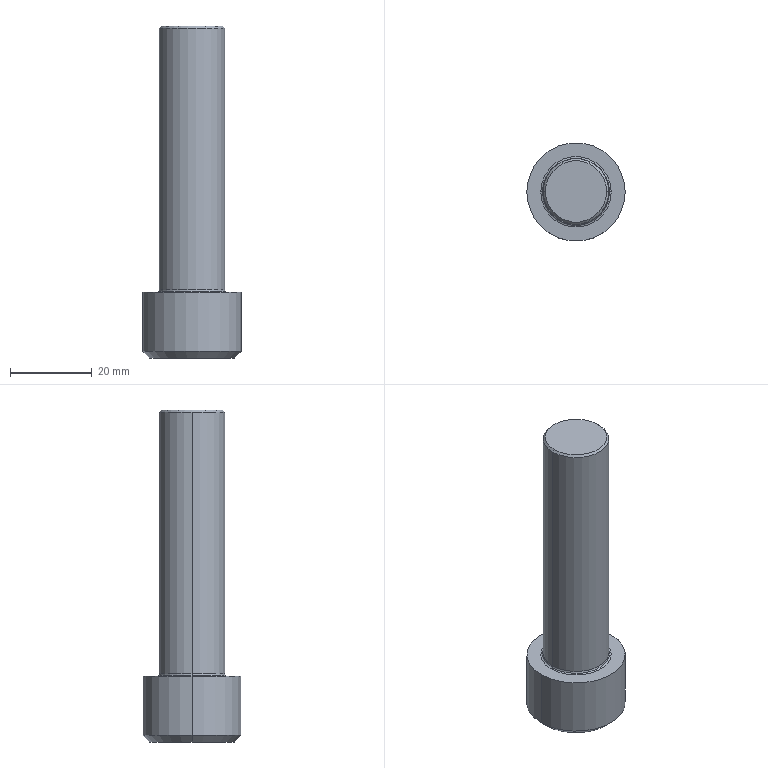Part | Creo | 1 solid | 23 faces | box 24 x 24 x 81 mm | volume 18544 mm3 | plane 9 | cone 6 | cylinder 4 | torus 4 | commonest cylinder face diameters 16 x2 24 x2
STEP:
#1=CARTESIAN_POINT('',(0.,0.,0.));
#2=DIRECTION('',(0.,0.,1.));
#3=DIRECTION('',(1.,0.,0.));
#4=AXIS2_PLACEMENT_3D('',#1,#2,#3);
#5=CARTESIAN_POINT('',(91.917,-8.,72.172));
#6=VERTEX_POINT('',#5);
#7=CARTESIAN_POINT('',(95.959,-1.,72.172));
#8=VERTEX_POINT('',#7);
#9=CARTESIAN_POINT('',(91.917,-8.,72.172));
#10=CARTESIAN_POINT('',(92.106,-7.673,72.281));
#11=CARTESIAN_POINT('',(92.484,-7.018,72.477));
#12=CARTESIAN_POINT('',(93.06,-6.021,72.689));
#13=CARTESIAN_POINT('',(93.642,-5.012,72.802));
#14=CARTESIAN_POINT('',(94.231,-3.992,72.802));
#15=CARTESIAN_POINT('',(94.814,-2.982,72.69));
#16=CARTESIAN_POINT('',(95.39,-1.986,72.478));
#17=CARTESIAN_POINT('',(95.769,-1.328,72.282));
#18=CARTESIAN_POINT('',(95.959,-1.,72.172));
#19=B_SPLINE_CURVE_WITH_KNOTS('',3,(#9,#10,#11,#12,#13,#14,#15,#16,#17,#18),.UNSPECIFIED.,.F.,.F.,(4,1,1,1,1,1,1,4),(0.,0.1429,0.2857,0.4286,0.5714,0.7143,0.8571,1.),.UNSPECIFIED.);
#20=EDGE_CURVE('',#6,#8,#19,.T.);
#21=ORIENTED_EDGE('',*,*,#20,.F.);
#22=CARTESIAN_POINT('',(100.,-8.,76.839));
#23=VERTEX_POINT('',#22);
#24=CARTESIAN_POINT('',(100.,-8.,76.839));
#25=DIRECTION('',(-0.866,0.,-0.5));
#26=VECTOR('',#25,9.333);
#27=LINE('',#24,#26);
#28=EDGE_CURVE('',#23,#6,#27,.T.);
#29=ORIENTED_EDGE('',*,*,#28,.F.);
#30=CARTESIAN_POINT('',(108.083,-8.,72.172));
#31=VERTEX_POINT('',#30);
#32=CARTESIAN_POINT('',(100.,-8.,76.839));
#33=DIRECTION('',(0.866,0.,-0.5));
#34=VECTOR('',#33,9.333);
#35=LINE('',#32,#34);
#36=EDGE_CURVE('',#23,#31,#35,.T.);
#37=ORIENTED_EDGE('',*,*,#36,.T.);
#38=CARTESIAN_POINT('',(104.041,-1.,72.172));
#39=VERTEX_POINT('',#38);
#40=CARTESIAN_POINT('',(104.041,-1.,72.172));
#41=CARTESIAN_POINT('',(104.23,-1.327,72.281));
#42=CARTESIAN_POINT('',(104.609,-1.982,72.477));
#43=CARTESIAN_POINT('',(105.184,-2.979,72.689));
#44=CARTESIAN_POINT('',(105.767,-3.988,72.802));
#45=CARTESIAN_POINT('',(106.356,-5.008,72.802));
#46=CARTESIAN_POINT('',(106.939,-6.018,72.69));
#47=CARTESIAN_POINT('',(107.514,-7.014,72.478));
#48=CARTESIAN_POINT('',(107.894,-7.672,72.282));
#49=CARTESIAN_POINT('',(108.083,-8.,72.172));
#50=B_SPLINE_CURVE_WITH_KNOTS('',3,(#40,#41,#42,#43,#44,#45,#46,#47,#48,#49),.UNSPECIFIED.,.F.,.F.,(4,1,1,1,1,1,1,4),(0.,0.1429,0.2857,0.4286,0.5714,0.7143,0.8571,1.),.UNSPECIFIED.);
#51=EDGE_CURVE('',#39,#31,#50,.T.);
#52=ORIENTED_EDGE('',*,*,#51,.F.);
#53=CARTESIAN_POINT('',(95.959,-1.,72.172));
#54=CARTESIAN_POINT('',(96.333,-1.,72.281));
#55=CARTESIAN_POINT('',(97.086,-1.,72.476));
#56=CARTESIAN_POINT('',(98.244,-1.,72.69));
#57=CARTESIAN_POINT('',(99.413,-1.,72.802));
#58=CARTESIAN_POINT('',(100.583,-1.,72.802));
#59=CARTESIAN_POINT('',(101.75,-1.,72.69));
#60=CARTESIAN_POINT('',(102.908,-1.,72.477));
#61=CARTESIAN_POINT('',(103.665,-1.,72.281));
#62=CARTESIAN_POINT('',(104.041,-1.,72.172));
#63=B_SPLINE_CURVE_WITH_KNOTS('',3,(#53,#54,#55,#56,#57,#58,#59,#60,#61,#62),.UNSPECIFIED.,.F.,.F.,(4,1,1,1,1,1,1,4),(0.,0.1429,0.2857,0.4286,0.5714,0.7143,0.8571,1.),.UNSPECIFIED.);
#64=EDGE_CURVE('',#8,#39,#63,.T.);
#65=ORIENTED_EDGE('',*,*,#64,.F.);
#66=EDGE_LOOP('',(#21,#29,#37,#52,#65));
#67=FACE_OUTER_BOUND('',#66,.F.);
#68=CARTESIAN_POINT('',(100.,-8.,74.459));
#69=DIRECTION('',(0.,0.,-1.));
#70=DIRECTION('',(-1.,0.,0.));
#71=AXIS2_PLACEMENT_3D('',#68,#69,#70);
#72=CONICAL_SURFACE('',#71,4.122,60.);
#73=ADVANCED_FACE('',(#67),#72,.F.);
#74=CARTESIAN_POINT('',(95.959,-1.,64.172));
#75=VERTEX_POINT('',#74);
#76=CARTESIAN_POINT('',(91.917,-8.,64.172));
#77=VERTEX_POINT('',#76);
#78=CARTESIAN_POINT('',(95.959,-1.,64.172));
#79=DIRECTION('',(-0.5,-0.866,0.));
#80=VECTOR('',#79,8.083);
#81=LINE('',#78,#80);
#82=EDGE_CURVE('',#75,#77,#81,.T.);
#83=ORIENTED_EDGE('',*,*,#82,.T.);
#84=CARTESIAN_POINT('',(91.917,-8.,64.172));
#85=DIRECTION('',(0.,0.,1.));
#86=VECTOR('',#85,8.);
#87=LINE('',#84,#86);
#88=EDGE_CURVE('',#77,#6,#87,.T.);
#89=ORIENTED_EDGE('',*,*,#88,.T.);
#90=ORIENTED_EDGE('',*,*,#20,.T.);
#91=CARTESIAN_POINT('',(95.959,-1.,64.172));
#92=DIRECTION('',(0.,0.,1.));
#93=VECTOR('',#92,8.);
#94=LINE('',#91,#93);
#95=EDGE_CURVE('',#75,#8,#94,.T.);
#96=ORIENTED_EDGE('',*,*,#95,.F.);
#97=EDGE_LOOP('',(#83,#89,#90,#96));
#98=FACE_OUTER_BOUND('',#97,.F.);
#99=CARTESIAN_POINT('',(95.959,-1.,72.172));
#100=DIRECTION('',(0.866,-0.5,0.));
#101=DIRECTION('',(-0.5,-0.866,0.));
#102=AXIS2_PLACEMENT_3D('',#99,#100,#101);
#103=PLANE('',#102);
#104=ADVANCED_FACE('',(#98),#103,.T.);
#105=CARTESIAN_POINT('',(89.6,-8.,64.172));
#106=VERTEX_POINT('',#105);
#107=CARTESIAN_POINT('',(110.4,-8.,64.172));
#108=VERTEX_POINT('',#107);
#109=CARTESIAN_POINT('',(100.,-8.,64.172));
#110=DIRECTION('',(0.,0.,-1.));
#111=DIRECTION('',(-1.,0.,0.));
#112=AXIS2_PLACEMENT_3D('',#109,#110,#111);
#113=CIRCLE('',#112,10.4);
#114=EDGE_CURVE('',#106,#108,#113,.T.);
#115=ORIENTED_EDGE('',*,*,#114,.F.);
#116=CARTESIAN_POINT('',(100.,-8.,64.172));
#117=DIRECTION('',(0.,0.,-1.));
#118=DIRECTION('',(1.,0.,0.));
#119=AXIS2_PLACEMENT_3D('',#116,#117,#118);
#120=CIRCLE('',#119,10.4);
#121=EDGE_CURVE('',#108,#106,#120,.T.);
#122=ORIENTED_EDGE('',*,*,#121,.F.);
#123=EDGE_LOOP('',(#115,#122));
#124=FACE_OUTER_BOUND('',#123,.F.);
#125=CARTESIAN_POINT('',(95.959,-15.,64.172));
#126=VERTEX_POINT('',#125);
#127=CARTESIAN_POINT('',(91.917,-8.,64.172));
#128=DIRECTION('',(0.5,-0.866,0.));
#129=VECTOR('',#128,8.083);
#130=LINE('',#127,#129);
#131=EDGE_CURVE('',#77,#126,#130,.T.);
#132=ORIENTED_EDGE('',*,*,#131,.F.);
#133=ORIENTED_EDGE('',*,*,#82,.F.);
#134=CARTESIAN_POINT('',(104.041,-1.,64.172));
#135=VERTEX_POINT('',#134);
#136=CARTESIAN_POINT('',(95.959,-1.,64.172));
#137=DIRECTION('',(1.,0.,0.));
#138=VECTOR('',#137,8.083);
#139=LINE('',#136,#138);
#140=EDGE_CURVE('',#75,#135,#139,.T.);
#141=ORIENTED_EDGE('',*,*,#140,.T.);
#142=CARTESIAN_POINT('',(108.083,-8.,64.172));
#143=VERTEX_POINT('',#142);
#144=CARTESIAN_POINT('',(108.083,-8.,64.172));
#145=DIRECTION('',(-0.5,0.866,0.));
#146=VECTOR('',#145,8.083);
#147=LINE('',#144,#146);
#148=EDGE_CURVE('',#143,#135,#147,.T.);
#149=ORIENTED_EDGE('',*,*,#148,.F.);
#150=CARTESIAN_POINT('',(104.041,-15.,64.172));
#151=VERTEX_POINT('',#150);
#152=CARTESIAN_POINT('',(104.041,-15.,64.172));
#153=DIRECTION('',(0.5,0.866,0.));
#154=VECTOR('',#153,8.083);
#155=LINE('',#152,#154);
#156=EDGE_CURVE('',#151,#143,#155,.T.);
#157=ORIENTED_EDGE('',*,*,#156,.F.);
#158=CARTESIAN_POINT('',(104.041,-15.,64.172));
#159=DIRECTION('',(-1.,0.,0.));
#160=VECTOR('',#159,8.083);
#161=LINE('',#158,#160);
#162=EDGE_CURVE('',#151,#126,#161,.T.);
#163=ORIENTED_EDGE('',*,*,#162,.T.);
#164=EDGE_LOOP('',(#132,#133,#141,#149,#157,#163));
#165=FACE_BOUND('',#164,.F.);
#166=CARTESIAN_POINT('',(100.,-8.,64.172));
#167=DIRECTION('',(0.,0.,-1.));
#168=DIRECTION('',(-1.,0.,0.));
#169=AXIS2_PLACEMENT_3D('',#166,#167,#168);
#170=PLANE('',#169);
#171=ADVANCED_FACE('',(#124,#165),#170,.T.);
#172=CARTESIAN_POINT('',(88.,-8.,65.772));
#173=VERTEX_POINT('',#172);
#174=CARTESIAN_POINT('',(112.,-8.,65.772));
#175=VERTEX_POINT('',#174);
#176=CARTESIAN_POINT('',(100.,-8.,65.772));
#177=DIRECTION('',(0.,0.,-1.));
#178=DIRECTION('',(-1.,0.,0.));
#179=AXIS2_PLACEMENT_3D('',#176,#177,#178);
#180=CIRCLE('',#179,12.);
#181=EDGE_CURVE('',#173,#175,#180,.T.);
#182=ORIENTED_EDGE('',*,*,#181,.F.);
#183=CARTESIAN_POINT('',(89.6,-8.,64.172));
#184=DIRECTION('',(-0.7071,0.,0.7071));
#185=VECTOR('',#184,2.263);
#186=LINE('',#183,#185);
#187=EDGE_CURVE('',#106,#173,#186,.T.);
#188=ORIENTED_EDGE('',*,*,#187,.F.);
#189=ORIENTED_EDGE('',*,*,#114,.T.);
#190=CARTESIAN_POINT('',(110.4,-8.,64.172));
#191=DIRECTION('',(0.7071,0.,0.7071));
#192=VECTOR('',#191,2.263);
#193=LINE('',#190,#192);
#194=EDGE_CURVE('',#108,#175,#193,.T.);
#195=ORIENTED_EDGE('',*,*,#194,.T.);
#196=EDGE_LOOP('',(#182,#188,#189,#195));
#197=FACE_OUTER_BOUND('',#196,.F.);
#198=CARTESIAN_POINT('',(100.,-8.,64.972));
#199=DIRECTION('',(0.,0.,1.));
#200=DIRECTION('',(1.,0.,0.));
#201=AXIS2_PLACEMENT_3D('',#198,#199,#200);
#202=CONICAL_SURFACE('',#201,11.2,45.);
#203=ADVANCED_FACE('',(#197),#202,.T.);
#204=ORIENTED_EDGE('',*,*,#181,.T.);
#205=CARTESIAN_POINT('',(112.,-8.,80.172));
#206=VERTEX_POINT('',#205);
#207=CARTESIAN_POINT('',(112.,-8.,80.172));
#208=DIRECTION('',(0.,0.,-1.));
#209=VECTOR('',#208,14.4);
#210=LINE('',#207,#209);
#211=EDGE_CURVE('',#206,#175,#210,.T.);
#212=ORIENTED_EDGE('',*,*,#211,.F.);
#213=CARTESIAN_POINT('',(88.,-8.,80.172));
#214=VERTEX_POINT('',#213);
#215=CARTESIAN_POINT('',(100.,-8.,80.172));
#216=DIRECTION('',(0.,0.,1.));
#217=DIRECTION('',(1.,0.,0.));
#218=AXIS2_PLACEMENT_3D('',#215,#216,#217);
#219=CIRCLE('',#218,12.);
#220=EDGE_CURVE('',#206,#214,#219,.T.);
#221=ORIENTED_EDGE('',*,*,#220,.T.);
#222=CARTESIAN_POINT('',(88.,-8.,80.172));
#223=DIRECTION('',(0.,0.,-1.));
#224=VECTOR('',#223,14.4);
#225=LINE('',#222,#224);
#226=EDGE_CURVE('',#214,#173,#225,.T.);
#227=ORIENTED_EDGE('',*,*,#226,.T.);
#228=EDGE_LOOP('',(#204,#212,#221,#227));
#229=FACE_OUTER_BOUND('',#228,.F.);
#230=CARTESIAN_POINT('',(100.,-8.,80.172));
#231=DIRECTION('',(0.,0.,-1.));
#232=DIRECTION('',(-1.,0.,0.));
#233=AXIS2_PLACEMENT_3D('',#230,#231,#232);
#234=CYLINDRICAL_SURFACE('',#233,12.);
#235=ADVANCED_FACE('',(#229),#234,.T.);
#236=CARTESIAN_POINT('',(100.,-8.,65.772));
#237=DIRECTION('',(0.,0.,-1.));
#238=DIRECTION('',(1.,0.,0.));
#239=AXIS2_PLACEMENT_3D('',#236,#237,#238);
#240=CIRCLE('',#239,12.);
#241=EDGE_CURVE('',#175,#173,#240,.T.);
#242=ORIENTED_EDGE('',*,*,#241,.T.);
#243=ORIENTED_EDGE('',*,*,#226,.F.);
#244=CARTESIAN_POINT('',(100.,-8.,80.172));
#245=DIRECTION('',(0.,0.,1.));
#246=DIRECTION('',(-1.,0.,0.));
#247=AXIS2_PLACEMENT_3D('',#244,#245,#246);
#248=CIRCLE('',#247,12.);
#249=EDGE_CURVE('',#214,#206,#248,.T.);
#250=ORIENTED_EDGE('',*,*,#249,.T.);
#251=ORIENTED_EDGE('',*,*,#211,.T.);
#252=EDGE_LOOP('',(#242,#243,#250,#251));
#253=FACE_OUTER_BOUND('',#252,.F.);
#254=CARTESIAN_POINT('',(100.,-8.,80.172));
#255=DIRECTION('',(0.,0.,-1.));
#256=DIRECTION('',(-1.,0.,0.));
#257=AXIS2_PLACEMENT_3D('',#254,#255,#256);
#258=CYLINDRICAL_SURFACE('',#257,12.);
#259=ADVANCED_FACE('',(#253),#258,.T.);
#260=ORIENTED_EDGE('',*,*,#241,.F.);
#261=ORIENTED_EDGE('',*,*,#194,.F.);
#262=ORIENTED_EDGE('',*,*,#121,.T.);
#263=ORIENTED_EDGE('',*,*,#187,.T.);
#264=EDGE_LOOP('',(#260,#261,#262,#263));
#265=FACE_OUTER_BOUND('',#264,.F.);
#266=CARTESIAN_POINT('',(100.,-8.,64.972));
#267=DIRECTION('',(0.,0.,1.));
#268=DIRECTION('',(1.,0.,0.));
#269=AXIS2_PLACEMENT_3D('',#266,#267,#268);
#270=CONICAL_SURFACE('',#269,11.2,45.);
#271=ADVANCED_FACE('',(#265),#270,.T.);
#272=ORIENTED_EDGE('',*,*,#249,.F.);
#273=ORIENTED_EDGE('',*,*,#220,.F.);
#274=EDGE_LOOP('',(#272,#273));
#275=FACE_OUTER_BOUND('',#274,.F.);
#276=CARTESIAN_POINT('',(91.4,-8.,80.172));
#277=VERTEX_POINT('',#276);
#278=CARTESIAN_POINT('',(108.6,-8.,80.172));
#279=VERTEX_POINT('',#278);
#280=CARTESIAN_POINT('',(100.,-8.,80.172));
#281=DIRECTION('',(0.,0.,-1.));
#282=DIRECTION('',(-1.,0.,0.));
#283=AXIS2_PLACEMENT_3D('',#280,#281,#282);
#284=CIRCLE('',#283,8.6);
#285=EDGE_CURVE('',#277,#279,#284,.T.);
#286=ORIENTED_EDGE('',*,*,#285,.F.);
#287=CARTESIAN_POINT('',(100.,-8.,80.172));
#288=DIRECTION('',(0.,0.,-1.));
#289=DIRECTION('',(1.,0.,0.));
#290=AXIS2_PLACEMENT_3D('',#287,#288,#289);
#291=CIRCLE('',#290,8.6);
#292=EDGE_CURVE('',#279,#277,#291,.T.);
#293=ORIENTED_EDGE('',*,*,#292,.F.);
#294=EDGE_LOOP('',(#286,#293));
#295=FACE_BOUND('',#294,.F.);
#296=CARTESIAN_POINT('',(100.,-8.,80.172));
#297=DIRECTION('',(0.,0.,-1.));
#298=DIRECTION('',(-1.,0.,0.));
#299=AXIS2_PLACEMENT_3D('',#296,#297,#298);
#300=PLANE('',#299);
#301=ADVANCED_FACE('',(#275,#295),#300,.F.);
#302=ORIENTED_EDGE('',*,*,#285,.T.);
#303=CARTESIAN_POINT('',(108.176,-8.,80.348));
#304=VERTEX_POINT('',#303);
#305=CARTESIAN_POINT('',(108.6,-8.,80.772));
#306=DIRECTION('',(0.,1.,0.));
#307=DIRECTION('',(0.,0.,-1.));
#308=AXIS2_PLACEMENT_3D('',#305,#306,#307);
#309=CIRCLE('',#308,0.6);
#310=EDGE_CURVE('',#279,#304,#309,.T.);
#311=ORIENTED_EDGE('',*,*,#310,.T.);
#312=CARTESIAN_POINT('',(91.824,-8.,80.348));
#313=VERTEX_POINT('',#312);
#314=CARTESIAN_POINT('',(100.,-8.,80.348));
#315=DIRECTION('',(0.,0.,-1.));
#316=DIRECTION('',(-1.,0.,0.));
#317=AXIS2_PLACEMENT_3D('',#314,#315,#316);
#318=CIRCLE('',#317,8.176);
#319=EDGE_CURVE('',#313,#304,#318,.T.);
#320=ORIENTED_EDGE('',*,*,#319,.F.);
#321=CARTESIAN_POINT('',(91.4,-8.,80.772));
#322=DIRECTION('',(0.,-1.,0.));
#323=DIRECTION('',(0.,0.,-1.));
#324=AXIS2_PLACEMENT_3D('',#321,#322,#323);
#325=CIRCLE('',#324,0.6);
#326=EDGE_CURVE('',#277,#313,#325,.T.);
#327=ORIENTED_EDGE('',*,*,#326,.F.);
#328=EDGE_LOOP('',(#302,#311,#320,#327));
#329=FACE_OUTER_BOUND('',#328,.F.);
#330=CARTESIAN_POINT('',(100.,-8.,80.772));
#331=DIRECTION('',(0.,0.,-1.));
#332=DIRECTION('',(-1.,0.,0.));
#333=AXIS2_PLACEMENT_3D('',#330,#331,#332);
#334=TOROIDAL_SURFACE('',#333,8.6,0.6);
#335=ADVANCED_FACE('',(#329),#334,.F.);
#336=ORIENTED_EDGE('',*,*,#292,.T.);
#337=ORIENTED_EDGE('',*,*,#326,.T.);
#338=CARTESIAN_POINT('',(100.,-8.,80.348));
#339=DIRECTION('',(0.,0.,-1.));
#340=DIRECTION('',(1.,0.,0.));
#341=AXIS2_PLACEMENT_3D('',#338,#339,#340);
#342=CIRCLE('',#341,8.176);
#343=EDGE_CURVE('',#304,#313,#342,.T.);
#344=ORIENTED_EDGE('',*,*,#343,.F.);
#345=ORIENTED_EDGE('',*,*,#310,.F.);
#346=EDGE_LOOP('',(#336,#337,#344,#345));
#347=FACE_OUTER_BOUND('',#346,.F.);
#348=CARTESIAN_POINT('',(100.,-8.,80.772));
#349=DIRECTION('',(0.,0.,-1.));
#350=DIRECTION('',(-1.,0.,0.));
#351=AXIS2_PLACEMENT_3D('',#348,#349,#350);
#352=TOROIDAL_SURFACE('',#351,8.6,0.6);
#353=ADVANCED_FACE('',(#347),#352,.F.);
#354=CARTESIAN_POINT('',(108.,-8.,80.772));
#355=VERTEX_POINT('',#354);
#356=CARTESIAN_POINT('',(92.,-8.,80.772));
#357=VERTEX_POINT('',#356);
#358=CARTESIAN_POINT('',(100.,-8.,80.772));
#359=DIRECTION('',(0.,0.,-1.));
#360=DIRECTION('',(1.,0.,0.));
#361=AXIS2_PLACEMENT_3D('',#358,#359,#360);
#362=CIRCLE('',#361,8.);
#363=EDGE_CURVE('',#355,#357,#362,.T.);
#364=ORIENTED_EDGE('',*,*,#363,.F.);
#365=CARTESIAN_POINT('',(108.6,-8.,80.772));
#366=DIRECTION('',(0.,1.,0.));
#367=DIRECTION('',(-0.7071,0.,-0.7071));
#368=AXIS2_PLACEMENT_3D('',#365,#366,#367);
#369=CIRCLE('',#368,0.6);
#370=EDGE_CURVE('',#304,#355,#369,.T.);
#371=ORIENTED_EDGE('',*,*,#370,.F.);
#372=ORIENTED_EDGE('',*,*,#343,.T.);
#373=CARTESIAN_POINT('',(91.4,-8.,80.772));
#374=DIRECTION('',(0.,-1.,0.));
#375=DIRECTION('',(0.7071,0.,-0.7071));
#376=AXIS2_PLACEMENT_3D('',#373,#374,#375);
#377=CIRCLE('',#376,0.6);
#378=EDGE_CURVE('',#313,#357,#377,.T.);
#379=ORIENTED_EDGE('',*,*,#378,.T.);
#380=EDGE_LOOP('',(#364,#371,#372,#379));
#381=FACE_OUTER_BOUND('',#380,.F.);
#382=CARTESIAN_POINT('',(100.,-8.,80.772));
#383=DIRECTION('',(0.,0.,-1.));
#384=DIRECTION('',(-1.,0.,0.));
#385=AXIS2_PLACEMENT_3D('',#382,#383,#384);
#386=TOROIDAL_SURFACE('',#385,8.6,0.6);
#387=ADVANCED_FACE('',(#381),#386,.F.);
#388=CARTESIAN_POINT('',(92.,-8.,144.673));
#389=VERTEX_POINT('',#388);
#390=CARTESIAN_POINT('',(108.,-8.,144.673));
#391=VERTEX_POINT('',#390);
#392=CARTESIAN_POINT('',(100.,-8.,144.673));
#393=DIRECTION('',(0.,0.,1.));
#394=DIRECTION('',(-1.,0.,0.));
#395=AXIS2_PLACEMENT_3D('',#392,#393,#394);
#396=CIRCLE('',#395,8.);
#397=EDGE_CURVE('',#389,#391,#396,.T.);
#398=ORIENTED_EDGE('',*,*,#397,.T.);
#399=CARTESIAN_POINT('',(108.,-8.,144.673));
#400=DIRECTION('',(0.,0.,-1.));
#401=VECTOR('',#400,63.9);
#402=LINE('',#399,#401);
#403=EDGE_CURVE('',#391,#355,#402,.T.);
#404=ORIENTED_EDGE('',*,*,#403,.T.);
#405=ORIENTED_EDGE('',*,*,#363,.T.);
#406=CARTESIAN_POINT('',(92.,-8.,144.673));
#407=DIRECTION('',(0.,0.,-1.));
#408=VECTOR('',#407,63.9);
#409=LINE('',#406,#408);
#410=EDGE_CURVE('',#389,#357,#409,.T.);
#411=ORIENTED_EDGE('',*,*,#410,.F.);
#412=EDGE_LOOP('',(#398,#404,#405,#411));
#413=FACE_OUTER_BOUND('',#412,.F.);
#414=CARTESIAN_POINT('',(100.,-8.,145.173));
#415=DIRECTION('',(0.,0.,-1.));
#416=DIRECTION('',(-1.,0.,0.));
#417=AXIS2_PLACEMENT_3D('',#414,#415,#416);
#418=CYLINDRICAL_SURFACE('',#417,8.);
#419=ADVANCED_FACE('',(#413),#418,.T.);
#420=CARTESIAN_POINT('',(92.5,-8.,145.173));
#421=VERTEX_POINT('',#420);
#422=CARTESIAN_POINT('',(107.5,-8.,145.173));
#423=VERTEX_POINT('',#422);
#424=CARTESIAN_POINT('',(100.,-8.,145.173));
#425=DIRECTION('',(0.,0.,1.));
#426=DIRECTION('',(-1.,0.,0.));
#427=AXIS2_PLACEMENT_3D('',#424,#425,#426);
#428=CIRCLE('',#427,7.5);
#429=EDGE_CURVE('',#421,#423,#428,.T.);
#430=ORIENTED_EDGE('',*,*,#429,.T.);
#431=CARTESIAN_POINT('',(107.5,-8.,145.173));
#432=DIRECTION('',(0.7071,0.,-0.7071));
#433=VECTOR('',#432,0.7071);
#434=LINE('',#431,#433);
#435=EDGE_CURVE('',#423,#391,#434,.T.);
#436=ORIENTED_EDGE('',*,*,#435,.T.);
#437=ORIENTED_EDGE('',*,*,#397,.F.);
#438=CARTESIAN_POINT('',(92.5,-8.,145.173));
#439=DIRECTION('',(-0.7071,0.,-0.7071));
#440=VECTOR('',#439,0.7071);
#441=LINE('',#438,#440);
#442=EDGE_CURVE('',#421,#389,#441,.T.);
#443=ORIENTED_EDGE('',*,*,#442,.F.);
#444=EDGE_LOOP('',(#430,#436,#437,#443));
#445=FACE_OUTER_BOUND('',#444,.F.);
#446=CARTESIAN_POINT('',(100.,-8.,144.923));
#447=DIRECTION('',(0.,0.,-1.));
#448=DIRECTION('',(-1.,0.,0.));
#449=AXIS2_PLACEMENT_3D('',#446,#447,#448);
#450=CONICAL_SURFACE('',#449,7.75,45.);
#451=ADVANCED_FACE('',(#445),#450,.T.);
#452=ORIENTED_EDGE('',*,*,#429,.F.);
#453=CARTESIAN_POINT('',(100.,-8.,145.173));
#454=DIRECTION('',(0.,0.,1.));
#455=DIRECTION('',(1.,0.,0.));
#456=AXIS2_PLACEMENT_3D('',#453,#454,#455);
#457=CIRCLE('',#456,7.5);
#458=EDGE_CURVE('',#423,#421,#457,.T.);
#459=ORIENTED_EDGE('',*,*,#458,.F.);
#460=EDGE_LOOP('',(#452,#459));
#461=FACE_OUTER_BOUND('',#460,.F.);
#462=CARTESIAN_POINT('',(100.,-8.,145.173));
#463=DIRECTION('',(0.,0.,-1.));
#464=DIRECTION('',(-1.,0.,0.));
#465=AXIS2_PLACEMENT_3D('',#462,#463,#464);
#466=PLANE('',#465);
#467=ADVANCED_FACE('',(#461),#466,.F.);
#468=ORIENTED_EDGE('',*,*,#458,.T.);
#469=ORIENTED_EDGE('',*,*,#442,.T.);
#470=CARTESIAN_POINT('',(100.,-8.,144.673));
#471=DIRECTION('',(0.,0.,1.));
#472=DIRECTION('',(1.,0.,0.));
#473=AXIS2_PLACEMENT_3D('',#470,#471,#472);
#474=CIRCLE('',#473,8.);
#475=EDGE_CURVE('',#391,#389,#474,.T.);
#476=ORIENTED_EDGE('',*,*,#475,.F.);
#477=ORIENTED_EDGE('',*,*,#435,.F.);
#478=EDGE_LOOP('',(#468,#469,#476,#477));
#479=FACE_OUTER_BOUND('',#478,.F.);
#480=CARTESIAN_POINT('',(100.,-8.,144.923));
#481=DIRECTION('',(0.,0.,-1.));
#482=DIRECTION('',(-1.,0.,0.));
#483=AXIS2_PLACEMENT_3D('',#480,#481,#482);
#484=CONICAL_SURFACE('',#483,7.75,45.);
#485=ADVANCED_FACE('',(#479),#484,.T.);
#486=ORIENTED_EDGE('',*,*,#475,.T.);
#487=ORIENTED_EDGE('',*,*,#410,.T.);
#488=CARTESIAN_POINT('',(100.,-8.,80.772));
#489=DIRECTION('',(0.,0.,-1.));
#490=DIRECTION('',(-1.,0.,0.));
#491=AXIS2_PLACEMENT_3D('',#488,#489,#490);
#492=CIRCLE('',#491,8.);
#493=EDGE_CURVE('',#357,#355,#492,.T.);
#494=ORIENTED_EDGE('',*,*,#493,.T.);
#495=ORIENTED_EDGE('',*,*,#403,.F.);
#496=EDGE_LOOP('',(#486,#487,#494,#495));
#497=FACE_OUTER_BOUND('',#496,.F.);
#498=CARTESIAN_POINT('',(100.,-8.,145.173));
#499=DIRECTION('',(0.,0.,-1.));
#500=DIRECTION('',(-1.,0.,0.));
#501=AXIS2_PLACEMENT_3D('',#498,#499,#500);
#502=CYLINDRICAL_SURFACE('',#501,8.);
#503=ADVANCED_FACE('',(#497),#502,.T.);
#504=ORIENTED_EDGE('',*,*,#493,.F.);
#505=ORIENTED_EDGE('',*,*,#378,.F.);
#506=ORIENTED_EDGE('',*,*,#319,.T.);
#507=ORIENTED_EDGE('',*,*,#370,.T.);
#508=EDGE_LOOP('',(#504,#505,#506,#507));
#509=FACE_OUTER_BOUND('',#508,.F.);
#510=CARTESIAN_POINT('',(100.,-8.,80.772));
#511=DIRECTION('',(0.,0.,-1.));
#512=DIRECTION('',(-1.,0.,0.));
#513=AXIS2_PLACEMENT_3D('',#510,#511,#512);
#514=TOROIDAL_SURFACE('',#513,8.6,0.6);
#515=ADVANCED_FACE('',(#509),#514,.F.);
#516=ORIENTED_EDGE('',*,*,#131,.T.);
#517=CARTESIAN_POINT('',(95.959,-15.,72.172));
#518=VERTEX_POINT('',#517);
#519=CARTESIAN_POINT('',(95.959,-15.,64.172));
#520=DIRECTION('',(0.,0.,1.));
#521=VECTOR('',#520,8.);
#522=LINE('',#519,#521);
#523=EDGE_CURVE('',#126,#518,#522,.T.);
#524=ORIENTED_EDGE('',*,*,#523,.T.);
#525=CARTESIAN_POINT('',(95.959,-15.,72.172));
#526=CARTESIAN_POINT('',(95.77,-14.673,72.281));
#527=CARTESIAN_POINT('',(95.391,-14.018,72.477));
#528=CARTESIAN_POINT('',(94.816,-13.021,72.689));
#529=CARTESIAN_POINT('',(94.233,-12.012,72.802));
#530=CARTESIAN_POINT('',(93.644,-10.992,72.802));
#531=CARTESIAN_POINT('',(93.061,-9.982,72.69));
#532=CARTESIAN_POINT('',(92.486,-8.986,72.478));
#533=CARTESIAN_POINT('',(92.106,-8.328,72.282));
#534=CARTESIAN_POINT('',(91.917,-8.,72.172));
#535=B_SPLINE_CURVE_WITH_KNOTS('',3,(#525,#526,#527,#528,#529,#530,#531,#532,#533,#534),.UNSPECIFIED.,.F.,.F.,(4,1,1,1,1,1,1,4),(0.,0.1429,0.2857,0.4286,0.5714,0.7143,0.8571,1.),.UNSPECIFIED.);
#536=EDGE_CURVE('',#518,#6,#535,.T.);
#537=ORIENTED_EDGE('',*,*,#536,.T.);
#538=ORIENTED_EDGE('',*,*,#88,.F.);
#539=EDGE_LOOP('',(#516,#524,#537,#538));
#540=FACE_OUTER_BOUND('',#539,.F.);
#541=CARTESIAN_POINT('',(91.917,-8.,72.172));
#542=DIRECTION('',(0.866,0.5,0.));
#543=DIRECTION('',(0.5,-0.866,0.));
#544=AXIS2_PLACEMENT_3D('',#541,#542,#543);
#545=PLANE('',#544);
#546=ADVANCED_FACE('',(#540),#545,.T.);
#547=ORIENTED_EDGE('',*,*,#162,.F.);
#548=CARTESIAN_POINT('',(104.041,-15.,72.172));
#549=VERTEX_POINT('',#548);
#550=CARTESIAN_POINT('',(104.041,-15.,64.172));
#551=DIRECTION('',(0.,0.,1.));
#552=VECTOR('',#551,8.);
#553=LINE('',#550,#552);
#554=EDGE_CURVE('',#151,#549,#553,.T.);
#555=ORIENTED_EDGE('',*,*,#554,.T.);
#556=CARTESIAN_POINT('',(104.041,-15.,72.172));
#557=CARTESIAN_POINT('',(103.665,-15.,72.281));
#558=CARTESIAN_POINT('',(102.908,-15.,72.477));
#559=CARTESIAN_POINT('',(101.75,-15.,72.69));
#560=CARTESIAN_POINT('',(100.583,-15.,72.802));
#561=CARTESIAN_POINT('',(99.413,-15.,72.802));
#562=CARTESIAN_POINT('',(98.244,-15.,72.69));
#563=CARTESIAN_POINT('',(97.086,-15.,72.476));
#564=CARTESIAN_POINT('',(96.333,-15.,72.281));
#565=CARTESIAN_POINT('',(95.959,-15.,72.172));
#566=B_SPLINE_CURVE_WITH_KNOTS('',3,(#556,#557,#558,#559,#560,#561,#562,#563,#564,#565),.UNSPECIFIED.,.F.,.F.,(4,1,1,1,1,1,1,4),(0.,0.1429,0.2857,0.4286,0.5714,0.7143,0.8571,1.),.UNSPECIFIED.);
#567=EDGE_CURVE('',#549,#518,#566,.T.);
#568=ORIENTED_EDGE('',*,*,#567,.T.);
#569=ORIENTED_EDGE('',*,*,#523,.F.);
#570=EDGE_LOOP('',(#547,#555,#568,#569));
#571=FACE_OUTER_BOUND('',#570,.F.);
#572=CARTESIAN_POINT('',(95.959,-15.,72.172));
#573=DIRECTION('',(0.,1.,0.));
#574=DIRECTION('',(0.,0.,-1.));
#575=AXIS2_PLACEMENT_3D('',#572,#573,#574);
#576=PLANE('',#575);
#577=ADVANCED_FACE('',(#571),#576,.T.);
#578=ORIENTED_EDGE('',*,*,#156,.T.);
#579=CARTESIAN_POINT('',(108.083,-8.,64.172));
#580=DIRECTION('',(0.,0.,1.));
#581=VECTOR('',#580,8.);
#582=LINE('',#579,#581);
#583=EDGE_CURVE('',#143,#31,#582,.T.);
#584=ORIENTED_EDGE('',*,*,#583,.T.);
#585=CARTESIAN_POINT('',(108.083,-8.,72.172));
#586=CARTESIAN_POINT('',(107.894,-8.328,72.282));
#587=CARTESIAN_POINT('',(107.514,-8.986,72.478));
#588=CARTESIAN_POINT('',(106.939,-9.982,72.69));
#589=CARTESIAN_POINT('',(106.356,-10.992,72.802));
#590=CARTESIAN_POINT('',(105.767,-12.012,72.802));
#591=CARTESIAN_POINT('',(105.184,-13.021,72.689));
#592=CARTESIAN_POINT('',(104.609,-14.018,72.477));
#593=CARTESIAN_POINT('',(104.23,-14.673,72.281));
#594=CARTESIAN_POINT('',(104.041,-15.,72.172));
#595=B_SPLINE_CURVE_WITH_KNOTS('',3,(#585,#586,#587,#588,#589,#590,#591,#592,#593,#594),.UNSPECIFIED.,.F.,.F.,(4,1,1,1,1,1,1,4),(0.,0.1429,0.2857,0.4286,0.5714,0.7143,0.8571,1.),.UNSPECIFIED.);
#596=EDGE_CURVE('',#31,#549,#595,.T.);
#597=ORIENTED_EDGE('',*,*,#596,.T.);
#598=ORIENTED_EDGE('',*,*,#554,.F.);
#599=EDGE_LOOP('',(#578,#584,#597,#598));
#600=FACE_OUTER_BOUND('',#599,.F.);
#601=CARTESIAN_POINT('',(104.041,-15.,72.172));
#602=DIRECTION('',(-0.866,0.5,0.));
#603=DIRECTION('',(0.5,0.866,0.));
#604=AXIS2_PLACEMENT_3D('',#601,#602,#603);
#605=PLANE('',#604);
#606=ADVANCED_FACE('',(#600),#605,.T.);
#607=ORIENTED_EDGE('',*,*,#148,.T.);
#608=CARTESIAN_POINT('',(104.041,-1.,64.172));
#609=DIRECTION('',(0.,0.,1.));
#610=VECTOR('',#609,8.);
#611=LINE('',#608,#610);
#612=EDGE_CURVE('',#135,#39,#611,.T.);
#613=ORIENTED_EDGE('',*,*,#612,.T.);
#614=ORIENTED_EDGE('',*,*,#51,.T.);
#615=ORIENTED_EDGE('',*,*,#583,.F.);
#616=EDGE_LOOP('',(#607,#613,#614,#615));
#617=FACE_OUTER_BOUND('',#616,.F.);
#618=CARTESIAN_POINT('',(108.083,-8.,72.172));
#619=DIRECTION('',(-0.866,-0.5,0.));
#620=DIRECTION('',(-0.5,0.866,0.));
#621=AXIS2_PLACEMENT_3D('',#618,#619,#620);
#622=PLANE('',#621);
#623=ADVANCED_FACE('',(#617),#622,.T.);
#624=ORIENTED_EDGE('',*,*,#140,.F.);
#625=ORIENTED_EDGE('',*,*,#95,.T.);
#626=ORIENTED_EDGE('',*,*,#64,.T.);
#627=ORIENTED_EDGE('',*,*,#612,.F.);
#628=EDGE_LOOP('',(#624,#625,#626,#627));
#629=FACE_OUTER_BOUND('',#628,.F.);
#630=CARTESIAN_POINT('',(104.041,-1.,72.172));
#631=DIRECTION('',(0.,-1.,0.));
#632=DIRECTION('',(0.,0.,1.));
#633=AXIS2_PLACEMENT_3D('',#630,#631,#632);
#634=PLANE('',#633);
#635=ADVANCED_FACE('',(#629),#634,.T.);
#636=ORIENTED_EDGE('',*,*,#596,.F.);
#637=ORIENTED_EDGE('',*,*,#36,.F.);
#638=ORIENTED_EDGE('',*,*,#28,.T.);
#639=ORIENTED_EDGE('',*,*,#536,.F.);
#640=ORIENTED_EDGE('',*,*,#567,.F.);
#641=EDGE_LOOP('',(#636,#637,#638,#639,#640));
#642=FACE_OUTER_BOUND('',#641,.F.);
#643=CARTESIAN_POINT('',(100.,-8.,74.459));
#644=DIRECTION('',(0.,0.,-1.));
#645=DIRECTION('',(-1.,0.,0.));
#646=AXIS2_PLACEMENT_3D('',#643,#644,#645);
#647=CONICAL_SURFACE('',#646,4.122,60.);
#648=ADVANCED_FACE('',(#642),#647,.F.);
#649=CLOSED_SHELL('',(#73,#104,#171,#203,#235,#259,#271,#301,#335,#353,#387,#419,#451,#467,#485,#503,#515,#546,#577,#606,#623,#635,#648));
#650=MANIFOLD_SOLID_BREP('',#649);
#651=(LENGTH_UNIT()NAMED_UNIT(*)SI_UNIT(.MILLI.,.METRE.));
#652=UNCERTAINTY_MEASURE_WITH_UNIT(LENGTH_MEASURE(0.008782),#651,'','');
#653=(NAMED_UNIT(*)PLANE_ANGLE_UNIT()SI_UNIT($,.RADIAN.));
#654=PLANE_ANGLE_MEASURE_WITH_UNIT(PLANE_ANGLE_MEASURE(0.01745),#653);
#655=(CONVERSION_BASED_UNIT('DEGREE',#654)NAMED_UNIT(*)PLANE_ANGLE_UNIT());
#656=(NAMED_UNIT(*)SI_UNIT($,.STERADIAN.)SOLID_ANGLE_UNIT());
#657=(GEOMETRIC_REPRESENTATION_CONTEXT(3)GLOBAL_UNCERTAINTY_ASSIGNED_CONTEXT((#652))GLOBAL_UNIT_ASSIGNED_CONTEXT((#651,#655,#656))REPRESENTATION_CONTEXT('',''));
#658=ADVANCED_BREP_SHAPE_REPRESENTATION('',(#4,#650),#657);